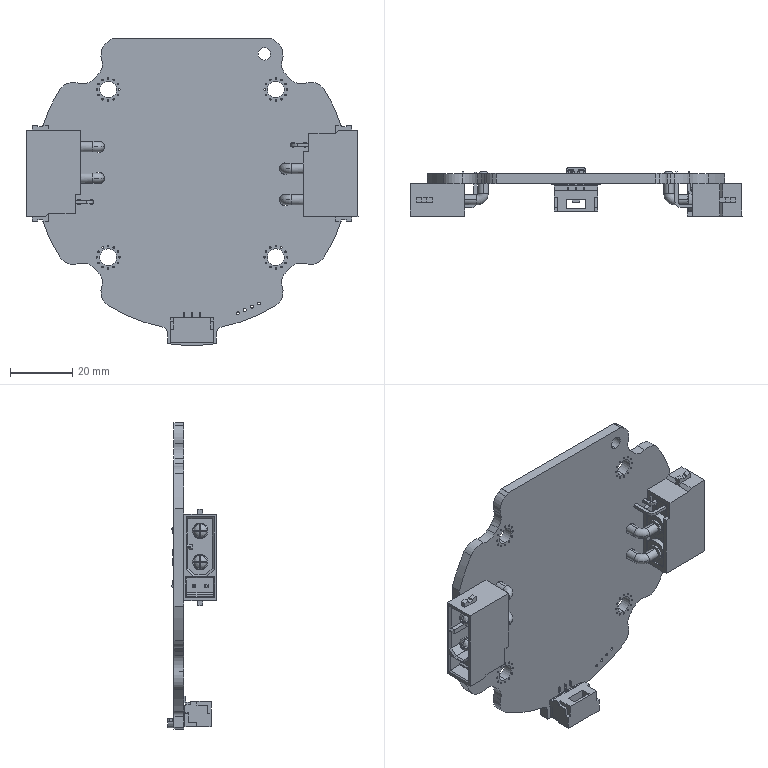Part | NX | features BREP 1 | 1 solid | 930 faces | box 106.4 x 15.6 x 98.256 mm | volume 29506 mm3 | plane 617 | cylinder 257 | cone 32 | spline 16 | torus 8 | commonest cylinder face diameters 0.508 x96 5 x18 3.2 x16 0.477 x12 1.2 x12 0.9 x8